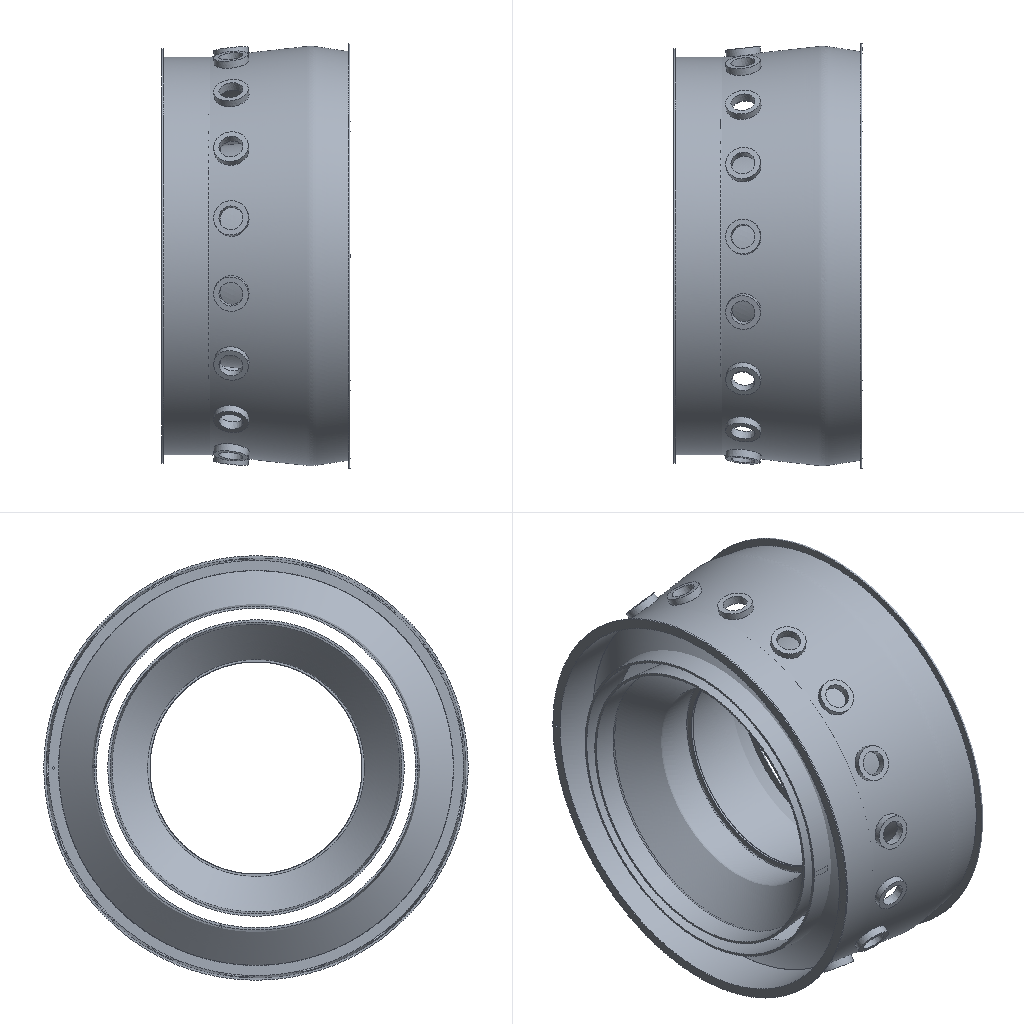Simulation study | ansys workbench
Set-up summary:
category,name,step,type,value,unit,region
solver,ansys_workbench
units,mm-N-s-tonne (MPa),,stated,"/units,MPA"
analysis,LS1,,modal,method=lanpcg; n_modes=4
load_step,LS1,LS1,modal
mesh,nodes,,,1043881
mesh,elements,,,524613
element_type,SOLID187,,,508745
element_type,CONTA174,,,7036
element_type,SOLID186,,,6528
element_type,TARGE170,,,2304
material,GH141,,E,216000
material,GH141,,nu,0.31
material,GH141,,density,8.27e-09,tonne mm^-3
material,GH141,,conductivity,8.37
material,GH141,,cte,1.054e-05
bc,Fixed Supports,model,fixed,[dofs=ALL],,_FIXEDSU
bc,Construct Remote Displacement,model,fixed,[dofs=UX],,node list
contact,Contact Region,,bonded (always),element=CONTA174
contact,contact 2,,bonded (always),element=CONTA174
contact,contact 3,,bonded (always),element=CONTA174
contact,contact 4,,bonded (always),element=CONTA174
named_set,_FIXEDSU,,node,6895
named_set,REMOTEDISPALL,,node,1
Ansys APDL input file, long lists of numbers shortened:
/batch
/config,noeldb,1     ! force off writing results to database
*get,_wallstrt,active,,time,wall
! ANSYS input file written by Workbench version 2021 R1
! File used for geometry attach:
/title,80--__ (D5)
! ****** Begin Custom Load Command Snippet ******
/COM, ACT Extensions:
/COM,     LSDYNA, 2021.1
/COM,
! ****** End   Custom Load Command Snippet ******
*DIM,_wb_ProjectScratch_dir,string,248
_wb_ProjectScratch_dir(1) = ''
*DIM,_wb_SolverFiles_dir,string,248
_wb_SolverFiles_dir(1) = ''
*DIM,_wb_userfiles_dir,string,248
_wb_userfiles_dir(1) = ''
/com,--- Data in consistent NMM units. See Solving Units in the help system for more information.
/units,MPA
/nopr
/wb,file,start              !  signify a WB generated input file
/prep7
! Turn off shape checking because checks already performed inside WB mesher.
! See help system for more information.
SHPP,OFF,,NOWARN
/nolist
etcon,set             ! allow ANSYS to choose best KEYOP's for 180x elements, resets any applicable keyopt to MAPDL defaults
/com,*********** Nodes for the whole assembly ***********
nblock,3,,1148263
(1i9,3e20.9e3)
        1    -2.909328663E+02    -6.564341511E+00     4.578700000E+02
! (1043875 more lines like these left out)
-1
/com,*********** Nodes for all Remote Points ***********
nblock,3
(1i9,3e20.9e3)
  1043877    -7.493286614E+01    -6.564353799E+00     2.143080415E+02
  1043878    -7.493286951E+01    -6.697121594E+00     2.143200000E+02
  1043879    -7.493286951E+01    -6.697121594E+00     2.143200000E+02
  1043880    -7.493286580E+01    -6.533767534E+00     2.143199692E+02
  1043881    -7.493286809E+01    -6.634512355E+00     2.143199882E+02
-1
/wb,elem,start            !  set before creation of elements
/com,*********** Elements for Body 1 "____9.24_\____9.24_" ***********
et,1,187
eblock,19,solid,,320859
(19i9)
        1        1        1        1        0        0        0        0       10        0   194415   420982   429274   496877   520848   545299   607590   545303   545309
! (641717 more lines like these left out)
-1
/com,*********** Elements for Body 2 "____0923_ (1)-0\____0923_ (1)" ***********
et,2,186
keyo,2,2,1          ! set full integration on SOLID186
eblock,19,solid,,6528
(19i9)
        2        2        2        2        0        0        0        0       20        0        1     1050     1051    13262    13261     7008     7007    13469    13470
! (13055 more lines like these left out)
-1
/com,*********** Elements for Body 3 "______9.22_\______9.22_" ***********
et,3,187
eblock,19,solid,,92984
(19i9)
        3        3        3        3        0        0        0        0       10        0    35420    54545   103924   108327   107989   161558   401449   161564   161563
! (185967 more lines like these left out)
-1
/com,*********** Elements for Body 4 "______9.24_\______9.24_" ***********
et,4,187
eblock,19,solid,,66011
(19i9)
        4        4        3        4        0        0        0        0       10        0   128404    55040   108946   103353   108755   164427   399349   164424   164426
! (132021 more lines like these left out)
-1
/com,*********** Elements for Body 5 "____0923_ (1)\____0923_ (1)" ***********
et,5,187
eblock,19,solid,,28891
(19i9)
        5        5        3        5        0        0        0        0       10        0     6529    48274    97425   107256    48526   115927   382662   115929   115926
! (57781 more lines like these left out)
-1
/wb,elem,end               !  done creating elements
/com,*********** Send User Defined Coordinate System(s) ***********
csys,0
toffst,273.15,  ! Temperature offset from absolute zero
/com,*********** Set Reference Temperature ***********
tref,22.
/wb,mat,start              !  starting to send materials
/com,*********** Send Materials ***********
Temperature = 'TEMP' ! Temperature
MP,DENS,1,8.27e-09,	! tonne mm^-3
MPTEMP,,,,,,,,
MPTEMP,1,100
MPTEMP,2,200
MPTEMP,3,300
MPTEMP,4,400
MPTEMP,5,500
MPTEMP,6,600
MPTEMP,7,700
MPTEMP,8,800
MPTEMP,9,900
MPDATA,EX,1, ,216000,210000,205000,200000,195000,188000,
MPDATA,EX,1, ,182000,175000,168000,	! tonne s^-2 mm^-1
MPTEMP,,,,,,,,
MPTEMP,,,,,,,,
MPTEMP,1,100
MPTEMP,2,200
MPTEMP,3,300
MPTEMP,4,400
MPTEMP,5,500
MPTEMP,6,600
MPTEMP,7,700
MPTEMP,8,800
MPTEMP,9,900
MPDATA,NUXY,1, ,0.31,0.31,0.31,0.31,0.31,0.31,
MPDATA,NUXY,1, ,0.31,0.31,0.31,
MPTEMP,,,,,,,,
MPTEMP,,,,,,,,
MPTEMP,1,100
MPTEMP,2,200
MPTEMP,3,300
MPTEMP,4,400
MPTEMP,5,500
MPTEMP,6,600
MPTEMP,7,700
MPTEMP,8,800
MPTEMP,9,900
MPDATA,ALPX,1, ,1.054e-05,1.169e-05,1.224e-05,1.278e-05,1.308e-05,1.348e-05,
MPDATA,ALPX,1, ,1.421e-05,1.497e-05,1.591e-05,	! C^-1
MPTEMP,,,,,,,,
MPTEMP,,,,,,,,
MPTEMP,1,100
MPTEMP,2,200
MPTEMP,3,300
MPTEMP,4,400
MPTEMP,5,500
MPTEMP,6,600
MPTEMP,7,700
MPTEMP,8,800
MPTEMP,9,900
MPDATA,KXX,1, ,8.37,10.47,12.56,15.07,17.17,19.56,
MPDATA,KXX,1, ,21.35,23.45,25.96,	! tonne mm s^-3 C^-1
MPTEMP,,,,,,,,
Temperature = 'TEMP' ! Temperature
MP,DENS,2,8.27e-09,	! tonne mm^-3
MPTEMP,,,,,,,,
MPTEMP,1,100
MPTEMP,2,200
MPTEMP,3,300
MPTEMP,4,400
MPTEMP,5,500
MPTEMP,6,600
MPTEMP,7,700
MPTEMP,8,800
MPTEMP,9,900
MPDATA,EX,2, ,216000,210000,205000,200000,195000,188000,
MPDATA,EX,2, ,182000,175000,168000,	! tonne s^-2 mm^-1
MPTEMP,,,,,,,,
MPTEMP,,,,,,,,
MPTEMP,1,100
MPTEMP,2,200
MPTEMP,3,300
MPTEMP,4,400
MPTEMP,5,500
MPTEMP,6,600
MPTEMP,7,700
MPTEMP,8,800
MPTEMP,9,900
MPDATA,NUXY,2, ,0.31,0.31,0.31,0.31,0.31,0.31,
MPDATA,NUXY,2, ,0.31,0.31,0.31,
MPTEMP,,,,,,,,
MPTEMP,,,,,,,,
MPTEMP,1,100
MPTEMP,2,200
MPTEMP,3,300
MPTEMP,4,400
MPTEMP,5,500
MPTEMP,6,600
MPTEMP,7,700
MPTEMP,8,800
MPTEMP,9,900
MPDATA,ALPX,2, ,1.054e-05,1.169e-05,1.224e-05,1.278e-05,1.308e-05,1.348e-05,
MPDATA,ALPX,2, ,1.421e-05,1.497e-05,1.591e-05,	! C^-1
MPTEMP,,,,,,,,
MPTEMP,,,,,,,,
MPTEMP,1,100
MPTEMP,2,200
MPTEMP,3,300
MPTEMP,4,400
MPTEMP,5,500
MPTEMP,6,600
MPTEMP,7,700
MPTEMP,8,800
MPTEMP,9,900
MPDATA,KXX,2, ,8.37,10.47,12.56,15.07,17.17,19.56,
MPDATA,KXX,2, ,21.35,23.45,25.96,	! tonne mm s^-3 C^-1
MPTEMP,,,,,,,,
Temperature = 'TEMP' ! Temperature
MP,DENS,3,8.27e-09,	! tonne mm^-3
MPTEMP,,,,,,,,
MPTEMP,1,100
MPTEMP,2,200
MPTEMP,3,300
MPTEMP,4,400
MPTEMP,5,500
MPTEMP,6,600
MPTEMP,7,700
MPTEMP,8,800
MPTEMP,9,900
MPDATA,EX,3, ,216000,210000,205000,200000,195000,188000,
MPDATA,EX,3, ,182000,175000,168000,	! tonne s^-2 mm^-1
MPTEMP,,,,,,,,
MPTEMP,,,,,,,,
MPTEMP,1,100
MPTEMP,2,200
MPTEMP,3,300
MPTEMP,4,400
MPTEMP,5,500
MPTEMP,6,600
MPTEMP,7,700
MPTEMP,8,800
MPTEMP,9,900
MPDATA,NUXY,3, ,0.31,0.31,0.31,0.31,0.31,0.31,
MPDATA,NUXY,3, ,0.31,0.31,0.31,
MPTEMP,,,,,,,,
MPTEMP,,,,,,,,
MPTEMP,1,100
MPTEMP,2,200
MPTEMP,3,300
MPTEMP,4,400
MPTEMP,5,500
MPTEMP,6,600
MPTEMP,7,700
MPTEMP,8,800
MPTEMP,9,900
MPDATA,ALPX,3, ,1.054e-05,1.169e-05,1.224e-05,1.278e-05,1.308e-05,1.348e-05,
MPDATA,ALPX,3, ,1.421e-05,1.497e-05,1.591e-05,	! C^-1
MPTEMP,,,,,,,,
MPTEMP,,,,,,,,
MPTEMP,1,100
MPTEMP,2,200
MPTEMP,3,300
MPTEMP,4,400
MPTEMP,5,500
MPTEMP,6,600
MPTEMP,7,700
MPTEMP,8,800
MPTEMP,9,900
MPDATA,KXX,3, ,8.37,10.47,12.56,15.07,17.17,19.56,
MPDATA,KXX,3, ,21.35,23.45,25.96,	! tonne mm s^-3 C^-1
MPTEMP,,,,,,,,
Temperature = 'TEMP' ! Temperature
MP,DENS,4,8.27e-09,	! tonne mm^-3
MPTEMP,,,,,,,,
MPTEMP,1,100
MPTEMP,2,200
MPTEMP,3,300
MPTEMP,4,400
MPTEMP,5,500
MPTEMP,6,600
MPTEMP,7,700
MPTEMP,8,800
MPTEMP,9,900
MPDATA,EX,4, ,216000,210000,205000,200000,195000,188000,
MPDATA,EX,4, ,182000,175000,168000,	! tonne s^-2 mm^-1
MPTEMP,,,,,,,,
MPTEMP,,,,,,,,
MPTEMP,1,100
MPTEMP,2,200
MPTEMP,3,300
MPTEMP,4,400
MPTEMP,5,500
MPTEMP,6,600
MPTEMP,7,700
MPTEMP,8,800
MPTEMP,9,900
MPDATA,NUXY,4, ,0.31,0.31,0.31,0.31,0.31,0.31,
MPDATA,NUXY,4, ,0.31,0.31,0.31,
MPTEMP,,,,,,,,
MPTEMP,,,,,,,,
MPTEMP,1,100
MPTEMP,2,200
MPTEMP,3,300
MPTEMP,4,400
MPTEMP,5,500
MPTEMP,6,600
MPTEMP,7,700
MPTEMP,8,800
MPTEMP,9,900
MPDATA,ALPX,4, ,1.054e-05,1.169e-05,1.224e-05,1.278e-05,1.308e-05,1.348e-05,
MPDATA,ALPX,4, ,1.421e-05,1.497e-05,1.591e-05,	! C^-1
MPTEMP,,,,,,,,
MPTEMP,,,,,,,,
MPTEMP,1,100
MPTEMP,2,200
MPTEMP,3,300
MPTEMP,4,400
MPTEMP,5,500
MPTEMP,6,600
MPTEMP,7,700
MPTEMP,8,800
MPTEMP,9,900
MPDATA,KXX,4, ,8.37,10.47,12.56,15.07,17.17,19.56,
MPDATA,KXX,4, ,21.35,23.45,25.96,	! tonne mm s^-3 C^-1
MPTEMP,,,,,,,,
Temperature = 'TEMP' ! Temperature
MP,DENS,5,8.27e-09,	! tonne mm^-3
MPTEMP,,,,,,,,
MPTEMP,1,100
MPTEMP,2,200
MPTEMP,3,300
MPTEMP,4,400
MPTEMP,5,500
MPTEMP,6,600
MPTEMP,7,700
MPTEMP,8,800
MPTEMP,9,900
MPDATA,EX,5, ,216000,210000,205000,200000,195000,188000,
MPDATA,EX,5, ,182000,175000,168000,	! tonne s^-2 mm^-1
MPTEMP,,,,,,,,
MPTEMP,,,,,,,,
MPTEMP,1,100
MPTEMP,2,200
MPTEMP,3,300
MPTEMP,4,400
MPTEMP,5,500
MPTEMP,6,600
MPTEMP,7,700
MPTEMP,8,800
MPTEMP,9,900
MPDATA,NUXY,5, ,0.31,0.31,0.31,0.31,0.31,0.31,
MPDATA,NUXY,5, ,0.31,0.31,0.31,
MPTEMP,,,,,,,,
MPTEMP,,,,,,,,
MPTEMP,1,100
MPTEMP,2,200
MPTEMP,3,300
MPTEMP,4,400
MPTEMP,5,500
MPTEMP,6,600
MPTEMP,7,700
MPTEMP,8,800
MPTEMP,9,900
MPDATA,ALPX,5, ,1.054e-05,1.169e-05,1.224e-05,1.278e-05,1.308e-05,1.348e-05,
MPDATA,ALPX,5, ,1.421e-05,1.497e-05,1.591e-05,	! C^-1
MPTEMP,,,,,,,,
MPTEMP,,,,,,,,
MPTEMP,1,100
MPTEMP,2,200
MPTEMP,3,300
MPTEMP,4,400
MPTEMP,5,500
MPTEMP,6,600
MPTEMP,7,700
MPTEMP,8,800
MPTEMP,9,900
MPDATA,KXX,5, ,8.37,10.47,12.56,15.07,17.17,19.56,
MPDATA,KXX,5, ,21.35,23.45,25.96,	! tonne mm s^-3 C^-1
MPTEMP,,,,,,,,
/wb,mat,end                !  done sending materials
!************************* Model Summary ********************
!____9.24_\____9.24_,	GH141,	matid,	1
!____0923_ (1)-0\____0923_ (1),	GH141,	matid,	2
!______9.22_\______9.22_,	GH141,	matid,	3
!______9.24_\______9.24_,	GH141,	matid,	4
!____0923_ (1)\____0923_ (1),	GH141,	matid,	5
!************************* End Model Summary ********************
! get the diagonal of the bounding box. Needed later for other things
*get,_xmin,node,,mnloc,x
*get,_ymin,node,,mnloc,y
*get,_zmin,node,,mnloc,z
*get,_xmax,node,,mxloc,x
*get,_ymax,node,,mxloc,y
*get,_zmax,node,,mxloc,z
_ASMDIAG=(_xmax-_xmin)*(_xmax-_xmin)+(_ymax-_ymin)*(_ymax-_ymin)+(_zmax-_zmin)*(_zmax-_zmin)
_ASMDIAG=SQRT(_ASMDIAG)
/wb,contact,start          !  starting to send contact
/com,*********** Create Contact "接触区域" ***********
/com,            Real Constant Set For Above Contact Is 7 & 6
*set,tid,7
*set,cid,6
r,tid
r,cid
et,tid,170
et,cid,174
eblock,10,,,768
(15i9)
   851575        7        7        7        0   423188   423189   423572   423572   564570   564576   423572   564572
! (767 more lines like these left out)
-1
eblock,10,,,768
(15i9)
   852343        6        6        6        0   423188   423189   423572   423572   564570   564576   423572   564572
! (767 more lines like these left out)
-1
eblock,10,,,1536
(15i9)
   853111        6        7        6        0     3446     3063     6901     6902    22949    22950    34083    24100
! (1535 more lines like these left out)
-1
eblock,10,,,1536
(15i9)
   854647        7        6        7        0     3446     3063     6901     6902    22949    22950    34083    24100
! (1535 more lines like these left out)
-1
keyo,cid,8,2               ! auto create asymmetric contact (from Program Controlled setting)
keyo,cid,10,0              ! adjust contact stiffness each NR iteration (from Program Controlled setting)
keyo,cid,12,5              ! bonded always
keyo,cid,18,1              ! small sliding turned on by application
keyo,cid,2,0               ! augmented Lagrange (from Program Controlled setting)
keyo,cid,4,0               ! on Gauss point (from Program Controlled setting)
keyo,cid,9,1               ! ignore initial gaps/penetration
keyo,cid,7,0               ! No Prediction
rmod,tid,3,10.      ! FKN
rmod,tid,5,0.       ! ICONT
rmod,tid,6,0.       ! PINB
rmod,tid,10,0.      ! CNOF
rmod,tid,12,0.      ! FKT
rmod,tid,36,113     ! WB DSID
rmod,cid,3,10.      ! FKN
rmod,cid,5,0.       ! ICONT
rmod,cid,6,0.       ! PINB
rmod,cid,10,0.      ! CNOF
rmod,cid,12,0.      ! FKT
rmod,cid,36,113     ! WB DSID
nsel,all
esel,all
/wb,contact,end            !  done creating contacts
/golist
/wb,load,start             !  starting to send loads
/com,*********** Fixed Supports ***********
CMBLOCK,_FIXEDSU,NODE,     6895
(8i10)
      6893      6894      6911      6912      6913      6914      6915      6916
! (861 more lines like these left out)
cmsel,s,_FIXEDSU
d,all,all
nsel,all
/com,*********** Create Remote Point "内部远程点 3" ***********
! -------- Remote Point Used by "远程位移" --------
*set,tid,9
*set,cid,8
et,cid,174
et,tid,170
keyo,tid,2,1               ! Don't fix the pilot node
keyo,tid,4,111111
keyo,cid,12,5              ! Bonded Contact
keyo,cid,4,1               ! Deformable RBE3 style load
keyo,cid,2,2               ! MPC style contact
eblock,10,,,2366
(15i9)
   856183        8        8        8        0    51746   106176    51747    51747   141736   141741    51747   141734
! (2365 more lines like these left out)
-1
*set,_npilot,1043881
_npilot173=_npilot
type,tid
mat ,cid
real,cid
tshape,pilo
en,858549,_npilot
tshape
/com,*********** Create Remote Point "远程点" ***********
*set,tid,11
*set,cid,10
et,cid,174
et,tid,170
keyo,tid,2,1               ! Don't fix the pilot node
keyo,tid,4,111111
keyo,cid,12,5              ! Bonded Contact
keyo,cid,4,1               ! Deformable RBE3 style load
keyo,cid,2,2               ! MPC style contact
eblock,10,,,900
(15i9)
   858550       10       10       10        0    51746   106176    51747    51747   141736   141741    51747   141734
! (899 more lines like these left out)
-1
*set,_npilot,1043877
_npilot87=_npilot
type,tid
mat ,cid
real,cid
tshape,pilo
en,859450,_npilot
tshape
/com,*********** Create Remote Point "远程点 2" ***********
*set,tid,13
*set,cid,12
et,cid,174
et,tid,170
keyo,tid,2,1               ! Don't fix the pilot node
keyo,tid,4,111111
keyo,cid,12,5              ! Bonded Contact
keyo,cid,4,1               ! Deformable RBE3 style load
keyo,cid,2,2               ! MPC style contact
eblock,10,,,1466
(15i9)
   859451       12       12       12        0   418454   418455   515807   515807   527672   527684   515807   527677
! (1465 more lines like these left out)
-1
*set,_npilot,1043878
_npilot89=_npilot
type,tid
mat ,cid
real,cid
tshape,pilo
en,860917,_npilot
tshape
/com,*********** Construct Remote Displacement ***********
*DIM,_loadvari172ux,TABLE,1,1,1,TIME,
! Time values
_loadvari172ux(1,0,1) = 1.
! Load values
_loadvari172ux(1,1,1) = 0.
d,1043881,ux,%_loadvari172ux%
/COM,*** Create a component for all remote displacements ***
CMBLOCK,REMOTEDISPALL,NODE,        1
(8i10)
   1043881
/gst,on,on
fini
*get,_numnode,node,0,count
*get,_numelem,elem,0,count
*get, _MAXELEMNUM, elem, 0, NUM, MAX
*get, _MAXNODENUM, node, 0, NUM, MAX
*get, _MAXELEMTYPE, etyp, 0, NUM, MAX
*get, _MAXREALCONST, real, 0, NUM, MAX
/go
/wb,load,end               !  done creating loads
/com,--- Number of total nodes = %_numnode%
/com,--- Number of contact elements = 9340
/com,--- Number of spring elements = 0
/com,--- Number of bearing elements = 0
/com,--- Number of solid elements = 515273
/com,--- Number of condensed parts = 0
/com,--- Number of total elements = %_numelem%
*get,_wallbsol,active,,time,wall
/solu
antype,2                   ! modal analysis
_thickRatio=  0     ! Ratio of thick parts in the model
modopt,lanpcg,4
eqslv,pcg
pcgopt,,,,,off         ! don't create file.full in order to save memory
msave,on
outres,erase
outres,all,none
outres,nsol,all
outres,etmp,all
mxpand                    ! default expand in case of complex solution
dmpopt,esav,no
dmpopt,emat,no
dmpopt,full,no
! *********** WB SOLVE COMMAND ***********
! check interactive state
*get,ANSINTER_,active,,int
*if,ANSINTER_,ne,0,then
/eof
*endif
solve
/com *************** Write FE CONNECTORS *********
CEWRITE,file,ce,,INTE
*get,_nmodalsolproc,active,0,numcpu
fini
/nopr
*get,_numnode,node,0,count
*get,_numelem,elem,0,count
*get, _MAXELEMNUM, elem, 0, NUM, MAX
*get, _MAXNODENUM, node, 0, NUM, MAX,,,INTERNAL
*get, _MAXELEMTYPE, etyp, 0, NUM, MAX
*get, _MAXREALCONST, real, 0, NUM, MAX
/gopr
*get,_wallasol,active,,time,wall
/post1
xmlo,ENCODING,ISO-8859-1
xmlo,parm
/xml,parm,xml
fini
/gopr
*get,_walldone,active,,time,wall
_preptime=(_wallbsol-_wallstrt)*3600
_solvtime=(_wallasol-_wallbsol)*3600
_posttime=(_walldone-_wallasol)*3600
_totaltim=(_walldone-_wallstrt)*3600
*get,_dlbratio,active,0,solu,dlbr
*get,_combtime,active,0,solu,comb
/com,--- Total number of nodes = %_numnode%
/com,--- Total number of elements = %_numelem%
/com,--- Element load balance ratio = %_dlbratio%
/com,--- Time to combine distributed files = %_combtime%
/wb,file,end               ! done with WB generated input
Results summary:
result,analyses[0].index,,,1
result,analyses[0].system,,,SYS-3
result,analyses[0].deck,,,deck.dat
result,analyses[0].solve_status,,,completed
result,analyses[0].analysis_type,,,modal
result,analyses[0].physics,,,mechanical
result,analyses[0].unit_system,,,"NMM: mm, ton, N, s, mV, mA, degC"
result,analyses[0].n_sets,,,4
result,analyses[0].modal_frequencies_hz[1],,,369.682
result,analyses[0].modal_frequencies_hz[2],,,369.854
result,analyses[0].modal_frequencies_hz[3],,,423.202
result,analyses[0].modal_frequencies_hz[4],,,423.221
result,geometry_export[0][0],,,1.step
result,geometry_export[0][1],,,ok
result,geometry_export[0][2],,,39
result,geometry_export[1][0],,,2.step
result,geometry_export[1][1],,,ok
result,geometry_export[1][2],,,5